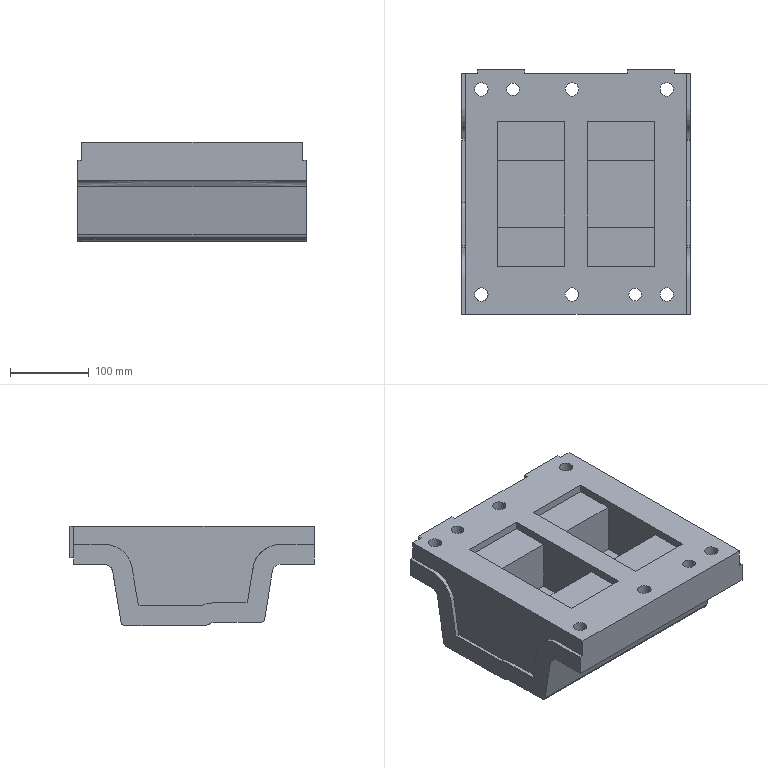Part | NX | features solid 2 | 1 solid | 123 faces | box 290 x 310 x 126.004 mm | volume 6972719 mm3 | plane 55 | spline 43 | cylinder 23 | torus 1 | cone 1 | commonest cylinder face diameters 17 x6 26 x6 12 x5 10 x3 16 x2 20 x1